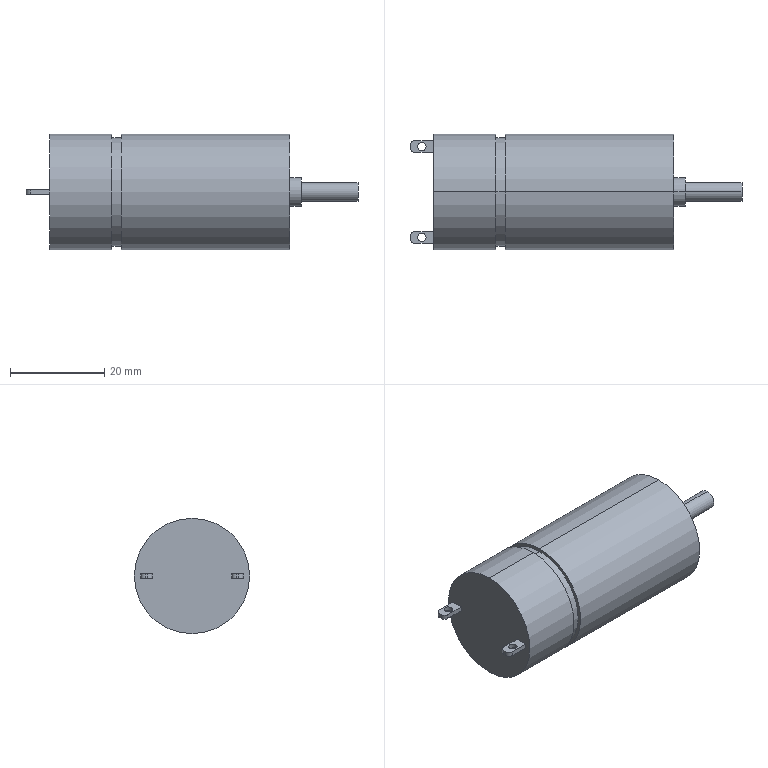Part | SolidWorks | features ICE 4, Extrusion 1, Fillet 1, RevCut 1 | 1 solid | 40 faces | box 70.5 x 24.5 x 24.5 mm | volume 24091 mm3 | cylinder 22 | plane 18 | commonest cylinder face diameters 1.8 x4 2 x4 3.2 x4 24.5 x4 4 x2 6 x2
STEP:
#1=CARTESIAN_POINT('',(46.,0.,-6.9));
#2=VERTEX_POINT('',#1);
#3=CARTESIAN_POINT('',(46.,0.,-10.1));
#4=VERTEX_POINT('',#3);
#5=CARTESIAN_POINT('',(46.,0.,-8.5));
#6=DIRECTION('',(1.,0.,0.));
#7=DIRECTION('',(0.,0.,-1.));
#8=AXIS2_PLACEMENT_3D('',#5,#6,#7);
#9=CIRCLE('',#8,1.6);
#10=EDGE_CURVE('',#2,#4,#9,.T.);
#11=ORIENTED_EDGE('',*,*,#10,.F.);
#12=CARTESIAN_POINT('',(51.,0.,-6.9));
#13=VERTEX_POINT('',#12);
#14=CARTESIAN_POINT('',(46.,0.,-6.9));
#15=DIRECTION('',(1.,0.,0.));
#16=VECTOR('',#15,1000.);
#17=LINE('',#14,#16);
#18=EDGE_CURVE('',#2,#13,#17,.T.);
#19=ORIENTED_EDGE('',*,*,#18,.T.);
#20=CARTESIAN_POINT('',(51.,0.,-10.1));
#21=VERTEX_POINT('',#20);
#22=CARTESIAN_POINT('',(51.,0.,-8.5));
#23=DIRECTION('',(1.,0.,0.));
#24=DIRECTION('',(0.,0.,-1.));
#25=AXIS2_PLACEMENT_3D('',#22,#23,#24);
#26=CIRCLE('',#25,1.6);
#27=EDGE_CURVE('',#13,#21,#26,.T.);
#28=ORIENTED_EDGE('',*,*,#27,.T.);
#29=CARTESIAN_POINT('',(46.,0.,-10.1));
#30=DIRECTION('',(1.,0.,0.));
#31=VECTOR('',#30,1000.);
#32=LINE('',#29,#31);
#33=EDGE_CURVE('',#4,#21,#32,.T.);
#34=ORIENTED_EDGE('',*,*,#33,.F.);
#35=EDGE_LOOP('',(#11,#19,#28,#34));
#36=FACE_OUTER_BOUND('',#35,.T.);
#37=CARTESIAN_POINT('',(46.,0.,-8.5));
#38=DIRECTION('',(1.,0.,0.));
#39=DIRECTION('',(0.,0.,-1.));
#40=AXIS2_PLACEMENT_3D('',#37,#38,#39);
#41=CYLINDRICAL_SURFACE('',#40,1.6);
#42=ADVANCED_FACE('',(#36),#41,.F.);
#43=CARTESIAN_POINT('',(46.,0.,10.1));
#44=VERTEX_POINT('',#43);
#45=CARTESIAN_POINT('',(46.,0.,6.9));
#46=VERTEX_POINT('',#45);
#47=CARTESIAN_POINT('',(46.,0.,8.5));
#48=DIRECTION('',(1.,0.,0.));
#49=DIRECTION('',(0.,0.,-1.));
#50=AXIS2_PLACEMENT_3D('',#47,#48,#49);
#51=CIRCLE('',#50,1.6);
#52=EDGE_CURVE('',#44,#46,#51,.T.);
#53=ORIENTED_EDGE('',*,*,#52,.F.);
#54=CARTESIAN_POINT('',(51.,0.,10.1));
#55=VERTEX_POINT('',#54);
#56=CARTESIAN_POINT('',(46.,0.,10.1));
#57=DIRECTION('',(1.,0.,0.));
#58=VECTOR('',#57,1000.);
#59=LINE('',#56,#58);
#60=EDGE_CURVE('',#44,#55,#59,.T.);
#61=ORIENTED_EDGE('',*,*,#60,.T.);
#62=CARTESIAN_POINT('',(51.,0.,6.9));
#63=VERTEX_POINT('',#62);
#64=CARTESIAN_POINT('',(51.,0.,8.5));
#65=DIRECTION('',(1.,0.,0.));
#66=DIRECTION('',(0.,0.,-1.));
#67=AXIS2_PLACEMENT_3D('',#64,#65,#66);
#68=CIRCLE('',#67,1.6);
#69=EDGE_CURVE('',#55,#63,#68,.T.);
#70=ORIENTED_EDGE('',*,*,#69,.T.);
#71=CARTESIAN_POINT('',(46.,0.,6.9));
#72=DIRECTION('',(1.,0.,0.));
#73=VECTOR('',#72,1000.);
#74=LINE('',#71,#73);
#75=EDGE_CURVE('',#46,#63,#74,.T.);
#76=ORIENTED_EDGE('',*,*,#75,.F.);
#77=EDGE_LOOP('',(#53,#61,#70,#76));
#78=FACE_OUTER_BOUND('',#77,.T.);
#79=CARTESIAN_POINT('',(46.,0.,8.5));
#80=DIRECTION('',(1.,0.,0.));
#81=DIRECTION('',(0.,0.,-1.));
#82=AXIS2_PLACEMENT_3D('',#79,#80,#81);
#83=CYLINDRICAL_SURFACE('',#82,1.6);
#84=ADVANCED_FACE('',(#78),#83,.F.);
#85=CARTESIAN_POINT('',(13.236,0.,-12.25));
#86=VERTEX_POINT('',#85);
#87=CARTESIAN_POINT('',(13.236,0.,12.25));
#88=VERTEX_POINT('',#87);
#89=CARTESIAN_POINT('',(13.236,0.,0.));
#90=DIRECTION('',(1.,0.,0.));
#91=DIRECTION('',(0.,0.,-1.));
#92=AXIS2_PLACEMENT_3D('',#89,#90,#91);
#93=CIRCLE('',#92,12.25);
#94=EDGE_CURVE('',#86,#88,#93,.T.);
#95=ORIENTED_EDGE('',*,*,#94,.F.);
#96=CARTESIAN_POINT('',(0.,0.,-12.25));
#97=VERTEX_POINT('',#96);
#98=CARTESIAN_POINT('',(51.,0.,-12.25));
#99=DIRECTION('',(-1.,0.,0.));
#100=VECTOR('',#99,1000.);
#101=LINE('',#98,#100);
#102=EDGE_CURVE('',#86,#97,#101,.T.);
#103=ORIENTED_EDGE('',*,*,#102,.T.);
#104=CARTESIAN_POINT('',(0.,0.,12.25));
#105=VERTEX_POINT('',#104);
#106=CARTESIAN_POINT('',(0.,0.,0.));
#107=DIRECTION('',(1.,0.,0.));
#108=DIRECTION('',(0.,0.,-1.));
#109=AXIS2_PLACEMENT_3D('',#106,#107,#108);
#110=CIRCLE('',#109,12.25);
#111=EDGE_CURVE('',#97,#105,#110,.T.);
#112=ORIENTED_EDGE('',*,*,#111,.T.);
#113=CARTESIAN_POINT('',(51.,0.,12.25));
#114=DIRECTION('',(-1.,0.,0.));
#115=VECTOR('',#114,1000.);
#116=LINE('',#113,#115);
#117=EDGE_CURVE('',#88,#105,#116,.T.);
#118=ORIENTED_EDGE('',*,*,#117,.F.);
#119=EDGE_LOOP('',(#95,#103,#112,#118));
#120=FACE_OUTER_BOUND('',#119,.T.);
#121=CARTESIAN_POINT('',(51.,0.,0.));
#122=DIRECTION('',(-1.,0.,0.));
#123=DIRECTION('',(0.,0.,1.));
#124=AXIS2_PLACEMENT_3D('',#121,#122,#123);
#125=CYLINDRICAL_SURFACE('',#124,12.25);
#126=ADVANCED_FACE('',(#120),#125,.T.);
#127=CARTESIAN_POINT('',(-3.4,9.654,0.5));
#128=VERTEX_POINT('',#127);
#129=CARTESIAN_POINT('',(-1.6,9.654,0.5));
#130=VERTEX_POINT('',#129);
#131=CARTESIAN_POINT('',(-2.5,9.654,0.5));
#132=DIRECTION('',(0.,0.,1.));
#133=DIRECTION('',(1.,0.,0.));
#134=AXIS2_PLACEMENT_3D('',#131,#132,#133);
#135=CIRCLE('',#134,0.9);
#136=EDGE_CURVE('',#128,#130,#135,.T.);
#137=ORIENTED_EDGE('',*,*,#136,.T.);
#138=CARTESIAN_POINT('',(-1.6,9.654,-0.5));
#139=VERTEX_POINT('',#138);
#140=CARTESIAN_POINT('',(-1.6,9.654,0.5));
#141=DIRECTION('',(0.,0.,-1.));
#142=VECTOR('',#141,1000.);
#143=LINE('',#140,#142);
#144=EDGE_CURVE('',#130,#139,#143,.T.);
#145=ORIENTED_EDGE('',*,*,#144,.T.);
#146=CARTESIAN_POINT('',(-3.4,9.654,-0.5));
#147=VERTEX_POINT('',#146);
#148=CARTESIAN_POINT('',(-2.5,9.654,-0.5));
#149=DIRECTION('',(0.,0.,1.));
#150=DIRECTION('',(1.,0.,0.));
#151=AXIS2_PLACEMENT_3D('',#148,#149,#150);
#152=CIRCLE('',#151,0.9);
#153=EDGE_CURVE('',#147,#139,#152,.T.);
#154=ORIENTED_EDGE('',*,*,#153,.F.);
#155=CARTESIAN_POINT('',(-3.4,9.654,0.5));
#156=DIRECTION('',(0.,0.,-1.));
#157=VECTOR('',#156,1000.);
#158=LINE('',#155,#157);
#159=EDGE_CURVE('',#128,#147,#158,.T.);
#160=ORIENTED_EDGE('',*,*,#159,.F.);
#161=EDGE_LOOP('',(#137,#145,#154,#160));
#162=FACE_OUTER_BOUND('',#161,.T.);
#163=CARTESIAN_POINT('',(-2.5,9.654,0.5));
#164=DIRECTION('',(0.,0.,-1.));
#165=DIRECTION('',(-1.,0.,0.));
#166=AXIS2_PLACEMENT_3D('',#163,#164,#165);
#167=CYLINDRICAL_SURFACE('',#166,0.9);
#168=ADVANCED_FACE('',(#162),#167,.F.);
#169=CARTESIAN_POINT('',(-3.4,-9.654,0.5));
#170=VERTEX_POINT('',#169);
#171=CARTESIAN_POINT('',(-1.6,-9.654,0.5));
#172=VERTEX_POINT('',#171);
#173=CARTESIAN_POINT('',(-2.5,-9.654,0.5));
#174=DIRECTION('',(0.,0.,1.));
#175=DIRECTION('',(-1.,0.,0.));
#176=AXIS2_PLACEMENT_3D('',#173,#174,#175);
#177=CIRCLE('',#176,0.9);
#178=EDGE_CURVE('',#170,#172,#177,.T.);
#179=ORIENTED_EDGE('',*,*,#178,.T.);
#180=CARTESIAN_POINT('',(-1.6,-9.654,-0.5));
#181=VERTEX_POINT('',#180);
#182=CARTESIAN_POINT('',(-1.6,-9.654,0.5));
#183=DIRECTION('',(0.,0.,-1.));
#184=VECTOR('',#183,1000.);
#185=LINE('',#182,#184);
#186=EDGE_CURVE('',#172,#181,#185,.T.);
#187=ORIENTED_EDGE('',*,*,#186,.T.);
#188=CARTESIAN_POINT('',(-3.4,-9.654,-0.5));
#189=VERTEX_POINT('',#188);
#190=CARTESIAN_POINT('',(-2.5,-9.654,-0.5));
#191=DIRECTION('',(0.,0.,1.));
#192=DIRECTION('',(-1.,0.,0.));
#193=AXIS2_PLACEMENT_3D('',#190,#191,#192);
#194=CIRCLE('',#193,0.9);
#195=EDGE_CURVE('',#189,#181,#194,.T.);
#196=ORIENTED_EDGE('',*,*,#195,.F.);
#197=CARTESIAN_POINT('',(-3.4,-9.654,0.5));
#198=DIRECTION('',(0.,0.,-1.));
#199=VECTOR('',#198,1000.);
#200=LINE('',#197,#199);
#201=EDGE_CURVE('',#170,#189,#200,.T.);
#202=ORIENTED_EDGE('',*,*,#201,.F.);
#203=EDGE_LOOP('',(#179,#187,#196,#202));
#204=FACE_OUTER_BOUND('',#203,.T.);
#205=CARTESIAN_POINT('',(-2.5,-9.654,0.5));
#206=DIRECTION('',(0.,0.,-1.));
#207=DIRECTION('',(-1.,0.,0.));
#208=AXIS2_PLACEMENT_3D('',#205,#206,#207);
#209=CYLINDRICAL_SURFACE('',#208,0.9);
#210=ADVANCED_FACE('',(#204),#209,.F.);
#211=CARTESIAN_POINT('',(15.236,0.,11.5));
#212=VERTEX_POINT('',#211);
#213=CARTESIAN_POINT('',(15.236,0.,-11.5));
#214=VERTEX_POINT('',#213);
#215=CARTESIAN_POINT('',(15.236,0.,0.));
#216=DIRECTION('',(-1.,0.,0.));
#217=DIRECTION('',(0.,0.,1.));
#218=AXIS2_PLACEMENT_3D('',#215,#216,#217);
#219=CIRCLE('',#218,11.5);
#220=EDGE_CURVE('',#212,#214,#219,.T.);
#221=ORIENTED_EDGE('',*,*,#220,.T.);
#222=CARTESIAN_POINT('',(13.236,0.,-11.5));
#223=VERTEX_POINT('',#222);
#224=CARTESIAN_POINT('',(-4.366,0.,-11.5));
#225=DIRECTION('',(-1.,0.,0.));
#226=VECTOR('',#225,1000.);
#227=LINE('',#224,#226);
#228=EDGE_CURVE('',#214,#223,#227,.T.);
#229=ORIENTED_EDGE('',*,*,#228,.T.);
#230=CARTESIAN_POINT('',(13.236,0.,11.5));
#231=VERTEX_POINT('',#230);
#232=CARTESIAN_POINT('',(13.236,0.,0.));
#233=DIRECTION('',(-1.,0.,0.));
#234=DIRECTION('',(0.,0.,1.));
#235=AXIS2_PLACEMENT_3D('',#232,#233,#234);
#236=CIRCLE('',#235,11.5);
#237=EDGE_CURVE('',#231,#223,#236,.T.);
#238=ORIENTED_EDGE('',*,*,#237,.F.);
#239=CARTESIAN_POINT('',(-4.366,0.,11.5));
#240=DIRECTION('',(-1.,0.,0.));
#241=VECTOR('',#240,1000.);
#242=LINE('',#239,#241);
#243=EDGE_CURVE('',#212,#231,#242,.T.);
#244=ORIENTED_EDGE('',*,*,#243,.F.);
#245=EDGE_LOOP('',(#221,#229,#238,#244));
#246=FACE_OUTER_BOUND('',#245,.T.);
#247=CARTESIAN_POINT('',(-4.366,0.,0.));
#248=DIRECTION('',(-1.,0.,0.));
#249=DIRECTION('',(0.,0.,1.));
#250=AXIS2_PLACEMENT_3D('',#247,#248,#249);
#251=CYLINDRICAL_SURFACE('',#250,11.5);
#252=ADVANCED_FACE('',(#246),#251,.T.);
#253=CARTESIAN_POINT('',(65.5,0.,-2.));
#254=VERTEX_POINT('',#253);
#255=CARTESIAN_POINT('',(65.5,0.,2.));
#256=VERTEX_POINT('',#255);
#257=CARTESIAN_POINT('',(65.5,0.,0.));
#258=DIRECTION('',(1.,0.,0.));
#259=DIRECTION('',(0.,0.,-1.));
#260=AXIS2_PLACEMENT_3D('',#257,#258,#259);
#261=CIRCLE('',#260,2.);
#262=EDGE_CURVE('',#254,#256,#261,.T.);
#263=ORIENTED_EDGE('',*,*,#262,.F.);
#264=CARTESIAN_POINT('',(53.5,0.,-2.));
#265=VERTEX_POINT('',#264);
#266=CARTESIAN_POINT('',(65.5,0.,-2.));
#267=DIRECTION('',(-1.,0.,0.));
#268=VECTOR('',#267,1000.);
#269=LINE('',#266,#268);
#270=EDGE_CURVE('',#254,#265,#269,.T.);
#271=ORIENTED_EDGE('',*,*,#270,.T.);
#272=CARTESIAN_POINT('',(53.5,0.,2.));
#273=VERTEX_POINT('',#272);
#274=CARTESIAN_POINT('',(53.5,0.,0.));
#275=DIRECTION('',(1.,0.,0.));
#276=DIRECTION('',(0.,0.,-1.));
#277=AXIS2_PLACEMENT_3D('',#274,#275,#276);
#278=CIRCLE('',#277,2.);
#279=EDGE_CURVE('',#265,#273,#278,.T.);
#280=ORIENTED_EDGE('',*,*,#279,.T.);
#281=CARTESIAN_POINT('',(65.5,0.,2.));
#282=DIRECTION('',(-1.,0.,0.));
#283=VECTOR('',#282,1000.);
#284=LINE('',#281,#283);
#285=EDGE_CURVE('',#256,#273,#284,.T.);
#286=ORIENTED_EDGE('',*,*,#285,.F.);
#287=EDGE_LOOP('',(#263,#271,#280,#286));
#288=FACE_OUTER_BOUND('',#287,.T.);
#289=CARTESIAN_POINT('',(65.5,0.,0.));
#290=DIRECTION('',(-1.,0.,0.));
#291=DIRECTION('',(0.,0.,1.));
#292=AXIS2_PLACEMENT_3D('',#289,#290,#291);
#293=CYLINDRICAL_SURFACE('',#292,2.);
#294=ADVANCED_FACE('',(#288),#293,.T.);
#295=CARTESIAN_POINT('',(53.5,0.,-3.));
#296=VERTEX_POINT('',#295);
#297=CARTESIAN_POINT('',(53.5,0.,3.));
#298=VERTEX_POINT('',#297);
#299=CARTESIAN_POINT('',(53.5,0.,0.));
#300=DIRECTION('',(1.,0.,0.));
#301=DIRECTION('',(0.,0.,-1.));
#302=AXIS2_PLACEMENT_3D('',#299,#300,#301);
#303=CIRCLE('',#302,3.);
#304=EDGE_CURVE('',#296,#298,#303,.T.);
#305=ORIENTED_EDGE('',*,*,#304,.F.);
#306=CARTESIAN_POINT('',(51.,0.,-3.));
#307=VERTEX_POINT('',#306);
#308=CARTESIAN_POINT('',(53.5,0.,-3.));
#309=DIRECTION('',(-1.,0.,0.));
#310=VECTOR('',#309,1000.);
#311=LINE('',#308,#310);
#312=EDGE_CURVE('',#296,#307,#311,.T.);
#313=ORIENTED_EDGE('',*,*,#312,.T.);
#314=CARTESIAN_POINT('',(51.,0.,3.));
#315=VERTEX_POINT('',#314);
#316=CARTESIAN_POINT('',(51.,0.,0.));
#317=DIRECTION('',(1.,0.,0.));
#318=DIRECTION('',(0.,0.,-1.));
#319=AXIS2_PLACEMENT_3D('',#316,#317,#318);
#320=CIRCLE('',#319,3.);
#321=EDGE_CURVE('',#307,#315,#320,.T.);
#322=ORIENTED_EDGE('',*,*,#321,.T.);
#323=CARTESIAN_POINT('',(53.5,0.,3.));
#324=DIRECTION('',(-1.,0.,0.));
#325=VECTOR('',#324,1000.);
#326=LINE('',#323,#325);
#327=EDGE_CURVE('',#298,#315,#326,.T.);
#328=ORIENTED_EDGE('',*,*,#327,.F.);
#329=EDGE_LOOP('',(#305,#313,#322,#328));
#330=FACE_OUTER_BOUND('',#329,.T.);
#331=CARTESIAN_POINT('',(53.5,0.,0.));
#332=DIRECTION('',(-1.,0.,0.));
#333=DIRECTION('',(0.,0.,1.));
#334=AXIS2_PLACEMENT_3D('',#331,#332,#333);
#335=CYLINDRICAL_SURFACE('',#334,3.);
#336=ADVANCED_FACE('',(#330),#335,.T.);
#337=CARTESIAN_POINT('',(51.,0.,-12.25));
#338=VERTEX_POINT('',#337);
#339=CARTESIAN_POINT('',(51.,0.,12.25));
#340=VERTEX_POINT('',#339);
#341=CARTESIAN_POINT('',(51.,0.,0.));
#342=DIRECTION('',(1.,0.,0.));
#343=DIRECTION('',(0.,0.,-1.));
#344=AXIS2_PLACEMENT_3D('',#341,#342,#343);
#345=CIRCLE('',#344,12.25);
#346=EDGE_CURVE('',#338,#340,#345,.T.);
#347=ORIENTED_EDGE('',*,*,#346,.F.);
#348=CARTESIAN_POINT('',(15.236,0.,-12.25));
#349=VERTEX_POINT('',#348);
#350=CARTESIAN_POINT('',(51.,0.,-12.25));
#351=DIRECTION('',(-1.,0.,0.));
#352=VECTOR('',#351,1000.);
#353=LINE('',#350,#352);
#354=EDGE_CURVE('',#338,#349,#353,.T.);
#355=ORIENTED_EDGE('',*,*,#354,.T.);
#356=CARTESIAN_POINT('',(15.236,0.,12.25));
#357=VERTEX_POINT('',#356);
#358=CARTESIAN_POINT('',(15.236,0.,0.));
#359=DIRECTION('',(-1.,0.,0.));
#360=DIRECTION('',(0.,0.,1.));
#361=AXIS2_PLACEMENT_3D('',#358,#359,#360);
#362=CIRCLE('',#361,12.25);
#363=EDGE_CURVE('',#357,#349,#362,.T.);
#364=ORIENTED_EDGE('',*,*,#363,.F.);
#365=CARTESIAN_POINT('',(51.,0.,12.25));
#366=DIRECTION('',(-1.,0.,0.));
#367=VECTOR('',#366,1000.);
#368=LINE('',#365,#367);
#369=EDGE_CURVE('',#340,#357,#368,.T.);
#370=ORIENTED_EDGE('',*,*,#369,.F.);
#371=EDGE_LOOP('',(#347,#355,#364,#370));
#372=FACE_OUTER_BOUND('',#371,.T.);
#373=CARTESIAN_POINT('',(51.,0.,0.));
#374=DIRECTION('',(-1.,0.,0.));
#375=DIRECTION('',(0.,0.,1.));
#376=AXIS2_PLACEMENT_3D('',#373,#374,#375);
#377=CYLINDRICAL_SURFACE('',#376,12.25);
#378=ADVANCED_FACE('',(#372),#377,.T.);
#379=ORIENTED_EDGE('',*,*,#354,.F.);
#380=CARTESIAN_POINT('',(51.,0.,0.));
#381=DIRECTION('',(1.,0.,0.));
#382=DIRECTION('',(0.,0.,-1.));
#383=AXIS2_PLACEMENT_3D('',#380,#381,#382);
#384=CIRCLE('',#383,12.25);
#385=EDGE_CURVE('',#340,#338,#384,.T.);
#386=ORIENTED_EDGE('',*,*,#385,.F.);
#387=ORIENTED_EDGE('',*,*,#369,.T.);
#388=CARTESIAN_POINT('',(15.236,0.,0.));
#389=DIRECTION('',(-1.,0.,0.));
#390=DIRECTION('',(0.,0.,1.));
#391=AXIS2_PLACEMENT_3D('',#388,#389,#390);
#392=CIRCLE('',#391,12.25);
#393=EDGE_CURVE('',#349,#357,#392,.T.);
#394=ORIENTED_EDGE('',*,*,#393,.F.);
#395=EDGE_LOOP('',(#379,#386,#387,#394));
#396=FACE_OUTER_BOUND('',#395,.T.);
#397=CARTESIAN_POINT('',(51.,0.,0.));
#398=DIRECTION('',(-1.,0.,0.));
#399=DIRECTION('',(0.,0.,1.));
#400=AXIS2_PLACEMENT_3D('',#397,#398,#399);
#401=CYLINDRICAL_SURFACE('',#400,12.25);
#402=ADVANCED_FACE('',(#396),#401,.T.);
#403=CARTESIAN_POINT('',(53.5,0.,0.));
#404=DIRECTION('',(1.,0.,0.));
#405=DIRECTION('',(0.,0.,-1.));
#406=AXIS2_PLACEMENT_3D('',#403,#404,#405);
#407=CIRCLE('',#406,3.);
#408=EDGE_CURVE('',#298,#296,#407,.T.);
#409=ORIENTED_EDGE('',*,*,#408,.T.);
#410=ORIENTED_EDGE('',*,*,#304,.T.);
#411=EDGE_LOOP('',(#409,#410));
#412=FACE_OUTER_BOUND('',#411,.T.);
#413=CARTESIAN_POINT('',(53.5,0.,0.));
#414=DIRECTION('',(1.,0.,0.));
#415=DIRECTION('',(0.,0.,-1.));
#416=AXIS2_PLACEMENT_3D('',#413,#414,#415);
#417=CIRCLE('',#416,2.);
#418=EDGE_CURVE('',#273,#265,#417,.T.);
#419=ORIENTED_EDGE('',*,*,#418,.F.);
#420=ORIENTED_EDGE('',*,*,#279,.F.);
#421=EDGE_LOOP('',(#419,#420));
#422=FACE_BOUND('',#421,.T.);
#423=CARTESIAN_POINT('',(53.5,0.,0.));
#424=DIRECTION('',(1.,0.,0.));
#425=DIRECTION('',(0.,0.,-1.));
#426=AXIS2_PLACEMENT_3D('',#423,#424,#425);
#427=PLANE('',#426);
#428=ADVANCED_FACE('',(#412,#422),#427,.T.);
#429=CARTESIAN_POINT('',(51.,0.,-8.5));
#430=DIRECTION('',(1.,0.,0.));
#431=DIRECTION('',(0.,0.,-1.));
#432=AXIS2_PLACEMENT_3D('',#429,#430,#431);
#433=CIRCLE('',#432,1.6);
#434=EDGE_CURVE('',#21,#13,#433,.T.);
#435=ORIENTED_EDGE('',*,*,#434,.F.);
#436=ORIENTED_EDGE('',*,*,#27,.F.);
#437=EDGE_LOOP('',(#435,#436));
#438=FACE_BOUND('',#437,.T.);
#439=CARTESIAN_POINT('',(51.,0.,8.5));
#440=DIRECTION('',(1.,0.,0.));
#441=DIRECTION('',(0.,0.,-1.));
#442=AXIS2_PLACEMENT_3D('',#439,#440,#441);
#443=CIRCLE('',#442,1.6);
#444=EDGE_CURVE('',#63,#55,#443,.T.);
#445=ORIENTED_EDGE('',*,*,#444,.F.);
#446=ORIENTED_EDGE('',*,*,#69,.F.);
#447=EDGE_LOOP('',(#445,#446));
#448=FACE_BOUND('',#447,.T.);
#449=ORIENTED_EDGE('',*,*,#385,.T.);
#450=ORIENTED_EDGE('',*,*,#346,.T.);
#451=EDGE_LOOP('',(#449,#450));
#452=FACE_OUTER_BOUND('',#451,.T.);
#453=CARTESIAN_POINT('',(51.,0.,0.));
#454=DIRECTION('',(1.,0.,0.));
#455=DIRECTION('',(0.,0.,-1.));
#456=AXIS2_PLACEMENT_3D('',#453,#454,#455);
#457=CIRCLE('',#456,3.);
#458=EDGE_CURVE('',#315,#307,#457,.T.);
#459=ORIENTED_EDGE('',*,*,#458,.F.);
#460=ORIENTED_EDGE('',*,*,#321,.F.);
#461=EDGE_LOOP('',(#459,#460));
#462=FACE_BOUND('',#461,.T.);
#463=CARTESIAN_POINT('',(51.,0.,0.));
#464=DIRECTION('',(1.,0.,0.));
#465=DIRECTION('',(0.,0.,-1.));
#466=AXIS2_PLACEMENT_3D('',#463,#464,#465);
#467=PLANE('',#466);
#468=ADVANCED_FACE('',(#438,#448,#452,#462),#467,.T.);
#469=ORIENTED_EDGE('',*,*,#312,.F.);
#470=ORIENTED_EDGE('',*,*,#408,.F.);
#471=ORIENTED_EDGE('',*,*,#327,.T.);
#472=ORIENTED_EDGE('',*,*,#458,.T.);
#473=EDGE_LOOP('',(#469,#470,#471,#472));
#474=FACE_OUTER_BOUND('',#473,.T.);
#475=CARTESIAN_POINT('',(53.5,0.,0.));
#476=DIRECTION('',(-1.,0.,0.));
#477=DIRECTION('',(0.,0.,1.));
#478=AXIS2_PLACEMENT_3D('',#475,#476,#477);
#479=CYLINDRICAL_SURFACE('',#478,3.);
#480=ADVANCED_FACE('',(#474),#479,.T.);
#481=ORIENTED_EDGE('',*,*,#270,.F.);
#482=CARTESIAN_POINT('',(65.5,0.,0.));
#483=DIRECTION('',(1.,0.,0.));
#484=DIRECTION('',(0.,0.,-1.));
#485=AXIS2_PLACEMENT_3D('',#482,#483,#484);
#486=CIRCLE('',#485,2.);
#487=EDGE_CURVE('',#256,#254,#486,.T.);
#488=ORIENTED_EDGE('',*,*,#487,.F.);
#489=ORIENTED_EDGE('',*,*,#285,.T.);
#490=ORIENTED_EDGE('',*,*,#418,.T.);
#491=EDGE_LOOP('',(#481,#488,#489,#490));
#492=FACE_OUTER_BOUND('',#491,.T.);
#493=CARTESIAN_POINT('',(65.5,0.,0.));
#494=DIRECTION('',(-1.,0.,0.));
#495=DIRECTION('',(0.,0.,1.));
#496=AXIS2_PLACEMENT_3D('',#493,#494,#495);
#497=CYLINDRICAL_SURFACE('',#496,2.);
#498=ADVANCED_FACE('',(#492),#497,.T.);
#499=ORIENTED_EDGE('',*,*,#487,.T.);
#500=ORIENTED_EDGE('',*,*,#262,.T.);
#501=EDGE_LOOP('',(#499,#500));
#502=FACE_OUTER_BOUND('',#501,.T.);
#503=CARTESIAN_POINT('',(65.5,0.,0.));
#504=DIRECTION('',(1.,0.,0.));
#505=DIRECTION('',(0.,0.,-1.));
#506=AXIS2_PLACEMENT_3D('',#503,#504,#505);
#507=PLANE('',#506);
#508=ADVANCED_FACE('',(#502),#507,.T.);
#509=ORIENTED_EDGE('',*,*,#220,.F.);
#510=CARTESIAN_POINT('',(15.236,0.,0.));
#511=DIRECTION('',(-1.,0.,0.));
#512=DIRECTION('',(0.,0.,1.));
#513=AXIS2_PLACEMENT_3D('',#510,#511,#512);
#514=CIRCLE('',#513,11.5);
#515=EDGE_CURVE('',#214,#212,#514,.T.);
#516=ORIENTED_EDGE('',*,*,#515,.F.);
#517=EDGE_LOOP('',(#509,#516));
#518=FACE_BOUND('',#517,.T.);
#519=ORIENTED_EDGE('',*,*,#363,.T.);
#520=ORIENTED_EDGE('',*,*,#393,.T.);
#521=EDGE_LOOP('',(#519,#520));
#522=FACE_OUTER_BOUND('',#521,.T.);
#523=CARTESIAN_POINT('',(15.236,15.,0.));
#524=DIRECTION('',(-1.,0.,0.));
#525=DIRECTION('',(0.,0.,1.));
#526=AXIS2_PLACEMENT_3D('',#523,#524,#525);
#527=PLANE('',#526);
#528=ADVANCED_FACE('',(#518,#522),#527,.T.);
#529=ORIENTED_EDGE('',*,*,#237,.T.);
#530=CARTESIAN_POINT('',(13.236,0.,0.));
#531=DIRECTION('',(-1.,0.,0.));
#532=DIRECTION('',(0.,0.,1.));
#533=AXIS2_PLACEMENT_3D('',#530,#531,#532);
#534=CIRCLE('',#533,11.5);
#535=EDGE_CURVE('',#223,#231,#534,.T.);
#536=ORIENTED_EDGE('',*,*,#535,.T.);
#537=EDGE_LOOP('',(#529,#536));
#538=FACE_BOUND('',#537,.T.);
#539=CARTESIAN_POINT('',(13.236,0.,0.));
#540=DIRECTION('',(1.,0.,0.));
#541=DIRECTION('',(0.,0.,-1.));
#542=AXIS2_PLACEMENT_3D('',#539,#540,#541);
#543=CIRCLE('',#542,12.25);
#544=EDGE_CURVE('',#88,#86,#543,.T.);
#545=ORIENTED_EDGE('',*,*,#544,.T.);
#546=ORIENTED_EDGE('',*,*,#94,.T.);
#547=EDGE_LOOP('',(#545,#546));
#548=FACE_OUTER_BOUND('',#547,.T.);
#549=CARTESIAN_POINT('',(13.236,15.,0.));
#550=DIRECTION('',(1.,0.,0.));
#551=DIRECTION('',(0.,0.,-1.));
#552=AXIS2_PLACEMENT_3D('',#549,#550,#551);
#553=PLANE('',#552);
#554=ADVANCED_FACE('',(#538,#548),#553,.T.);
#555=ORIENTED_EDGE('',*,*,#228,.F.);
#556=ORIENTED_EDGE('',*,*,#515,.T.);
#557=ORIENTED_EDGE('',*,*,#243,.T.);
#558=ORIENTED_EDGE('',*,*,#535,.F.);
#559=EDGE_LOOP('',(#555,#556,#557,#558));
#560=FACE_OUTER_BOUND('',#559,.T.);
#561=CARTESIAN_POINT('',(-4.366,0.,0.));
#562=DIRECTION('',(-1.,0.,0.));
#563=DIRECTION('',(0.,0.,1.));
#564=AXIS2_PLACEMENT_3D('',#561,#562,#563);
#565=CYLINDRICAL_SURFACE('',#564,11.5);
#566=ADVANCED_FACE('',(#560),#565,.T.);
#567=ORIENTED_EDGE('',*,*,#186,.F.);
#568=CARTESIAN_POINT('',(-2.5,-9.654,0.5));
#569=DIRECTION('',(0.,0.,1.));
#570=DIRECTION('',(-1.,0.,0.));
#571=AXIS2_PLACEMENT_3D('',#568,#569,#570);
#572=CIRCLE('',#571,0.9);
#573=EDGE_CURVE('',#172,#170,#572,.T.);
#574=ORIENTED_EDGE('',*,*,#573,.T.);
#575=ORIENTED_EDGE('',*,*,#201,.T.);
#576=CARTESIAN_POINT('',(-2.5,-9.654,-0.5));
#577=DIRECTION('',(0.,0.,1.));
#578=DIRECTION('',(-1.,0.,0.));
#579=AXIS2_PLACEMENT_3D('',#576,#577,#578);
#580=CIRCLE('',#579,0.9);
#581=EDGE_CURVE('',#181,#189,#580,.T.);
#582=ORIENTED_EDGE('',*,*,#581,.F.);
#583=EDGE_LOOP('',(#567,#574,#575,#582));
#584=FACE_OUTER_BOUND('',#583,.T.);
#585=CARTESIAN_POINT('',(-2.5,-9.654,0.5));
#586=DIRECTION('',(0.,0.,-1.));
#587=DIRECTION('',(-1.,0.,0.));
#588=AXIS2_PLACEMENT_3D('',#585,#586,#587);
#589=CYLINDRICAL_SURFACE('',#588,0.9);
#590=ADVANCED_FACE('',(#584),#589,.F.);
#591=CARTESIAN_POINT('',(-4.,-8.404,0.5));
#592=VERTEX_POINT('',#591);
#593=CARTESIAN_POINT('',(-5.,-9.404,0.5));
#594=VERTEX_POINT('',#593);
#595=CARTESIAN_POINT('',(-4.,-9.404,0.5));
#596=DIRECTION('',(0.,0.,1.));
#597=DIRECTION('',(-1.,0.,0.));
#598=AXIS2_PLACEMENT_3D('',#595,#596,#597);
#599=CIRCLE('',#598,1.);
#600=EDGE_CURVE('',#592,#594,#599,.T.);
#601=ORIENTED_EDGE('',*,*,#600,.F.);
#602=CARTESIAN_POINT('',(-4.,-8.404,-0.5));
#603=VERTEX_POINT('',#602);
#604=CARTESIAN_POINT('',(-4.,-8.404,0.5));
#605=DIRECTION('',(0.,0.,1.));
#606=VECTOR('',#605,1000.);
#607=LINE('',#604,#606);
#608=EDGE_CURVE('',#603,#592,#607,.T.);
#609=ORIENTED_EDGE('',*,*,#608,.F.);
#610=CARTESIAN_POINT('',(-5.,-9.404,-0.5));
#611=VERTEX_POINT('',#610);
#612=CARTESIAN_POINT('',(-4.,-9.404,-0.5));
#613=DIRECTION('',(0.,0.,-1.));
#614=DIRECTION('',(-1.,0.,0.));
#615=AXIS2_PLACEMENT_3D('',#612,#613,#614);
#616=CIRCLE('',#615,1.);
#617=EDGE_CURVE('',#611,#603,#616,.T.);
#618=ORIENTED_EDGE('',*,*,#617,.F.);
#619=CARTESIAN_POINT('',(-5.,-9.404,0.5));
#620=DIRECTION('',(0.,0.,-1.));
#621=VECTOR('',#620,1000.);
#622=LINE('',#619,#621);
#623=EDGE_CURVE('',#594,#611,#622,.T.);
#624=ORIENTED_EDGE('',*,*,#623,.F.);
#625=EDGE_LOOP('',(#601,#609,#618,#624));
#626=FACE_OUTER_BOUND('',#625,.T.);
#627=CARTESIAN_POINT('',(-4.,-9.404,0.5));
#628=DIRECTION('',(0.,0.,-1.));
#629=DIRECTION('',(-1.,0.,0.));
#630=AXIS2_PLACEMENT_3D('',#627,#628,#629);
#631=CYLINDRICAL_SURFACE('',#630,1.);
#632=ADVANCED_FACE('',(#626),#631,.T.);
#633=CARTESIAN_POINT('',(-5.,-9.904,0.5));
#634=VERTEX_POINT('',#633);
#635=CARTESIAN_POINT('',(-5.,-10.904,0.5));
#636=DIRECTION('',(0.,-1.,0.));
#637=VECTOR('',#636,1000.);
#638=LINE('',#635,#637);
#639=EDGE_CURVE('',#594,#634,#638,.T.);
#640=ORIENTED_EDGE('',*,*,#639,.F.);
#641=ORIENTED_EDGE('',*,*,#623,.T.);
#642=CARTESIAN_POINT('',(-5.,-9.904,-0.5));
#643=VERTEX_POINT('',#642);
#644=CARTESIAN_POINT('',(-5.,-10.904,-0.5));
#645=DIRECTION('',(0.,-1.,0.));
#646=VECTOR('',#645,1000.);
#647=LINE('',#644,#646);
#648=EDGE_CURVE('',#611,#643,#647,.T.);
#649=ORIENTED_EDGE('',*,*,#648,.T.);
#650=CARTESIAN_POINT('',(-5.,-9.904,0.5));
#651=DIRECTION('',(0.,0.,1.));
#652=VECTOR('',#651,1000.);
#653=LINE('',#650,#652);
#654=EDGE_CURVE('',#643,#634,#653,.T.);
#655=ORIENTED_EDGE('',*,*,#654,.T.);
#656=EDGE_LOOP('',(#640,#641,#649,#655));
#657=FACE_OUTER_BOUND('',#656,.T.);
#658=CARTESIAN_POINT('',(-5.,-10.904,0.5));
#659=DIRECTION('',(1.,0.,0.));
#660=DIRECTION('',(0.,1.,0.));
#661=AXIS2_PLACEMENT_3D('',#658,#659,#660);
#662=PLANE('',#661);
#663=ADVANCED_FACE('',(#657),#662,.F.);
#664=CARTESIAN_POINT('',(-4.,-10.904,0.5));
#665=VERTEX_POINT('',#664);
#666=CARTESIAN_POINT('',(-4.,-9.904,0.5));
#667=DIRECTION('',(0.,0.,1.));
#668=DIRECTION('',(-1.,0.,0.));
#669=AXIS2_PLACEMENT_3D('',#666,#667,#668);
#670=CIRCLE('',#669,1.);
#671=EDGE_CURVE('',#634,#665,#670,.T.);
#672=ORIENTED_EDGE('',*,*,#671,.F.);
#673=ORIENTED_EDGE('',*,*,#654,.F.);
#674=CARTESIAN_POINT('',(-4.,-10.904,-0.5));
#675=VERTEX_POINT('',#674);
#676=CARTESIAN_POINT('',(-4.,-9.904,-0.5));
#677=DIRECTION('',(0.,0.,-1.));
#678=DIRECTION('',(-1.,0.,0.));
#679=AXIS2_PLACEMENT_3D('',#676,#677,#678);
#680=CIRCLE('',#679,1.);
#681=EDGE_CURVE('',#675,#643,#680,.T.);
#682=ORIENTED_EDGE('',*,*,#681,.F.);
#683=CARTESIAN_POINT('',(-4.,-10.904,0.5));
#684=DIRECTION('',(0.,0.,-1.));
#685=VECTOR('',#684,1000.);
#686=LINE('',#683,#685);
#687=EDGE_CURVE('',#665,#675,#686,.T.);
#688=ORIENTED_EDGE('',*,*,#687,.F.);
#689=EDGE_LOOP('',(#672,#673,#682,#688));
#690=FACE_OUTER_BOUND('',#689,.T.);
#691=CARTESIAN_POINT('',(-4.,-9.904,0.5));
#692=DIRECTION('',(0.,0.,-1.));
#693=DIRECTION('',(-1.,0.,0.));
#694=AXIS2_PLACEMENT_3D('',#691,#692,#693);
#695=CYLINDRICAL_SURFACE('',#694,1.);
#696=ADVANCED_FACE('',(#690),#695,.T.);
#697=ORIENTED_EDGE('',*,*,#144,.F.);
#698=CARTESIAN_POINT('',(-2.5,9.654,0.5));
#699=DIRECTION('',(0.,0.,1.));
#700=DIRECTION('',(1.,0.,0.));
#701=AXIS2_PLACEMENT_3D('',#698,#699,#700);
#702=CIRCLE('',#701,0.9);
#703=EDGE_CURVE('',#130,#128,#702,.T.);
#704=ORIENTED_EDGE('',*,*,#703,.T.);
#705=ORIENTED_EDGE('',*,*,#159,.T.);
#706=CARTESIAN_POINT('',(-2.5,9.654,-0.5));
#707=DIRECTION('',(0.,0.,1.));
#708=DIRECTION('',(1.,0.,0.));
#709=AXIS2_PLACEMENT_3D('',#706,#707,#708);
#710=CIRCLE('',#709,0.9);
#711=EDGE_CURVE('',#139,#147,#710,.T.);
#712=ORIENTED_EDGE('',*,*,#711,.F.);
#713=EDGE_LOOP('',(#697,#704,#705,#712));
#714=FACE_OUTER_BOUND('',#713,.T.);
#715=CARTESIAN_POINT('',(-2.5,9.654,0.5));
#716=DIRECTION('',(0.,0.,-1.));
#717=DIRECTION('',(-1.,0.,0.));
#718=AXIS2_PLACEMENT_3D('',#715,#716,#717);
#719=CYLINDRICAL_SURFACE('',#718,0.9);
#720=ADVANCED_FACE('',(#714),#719,.F.);
#721=CARTESIAN_POINT('',(-5.,9.404,0.5));
#722=VERTEX_POINT('',#721);
#723=CARTESIAN_POINT('',(-4.,8.404,0.5));
#724=VERTEX_POINT('',#723);
#725=CARTESIAN_POINT('',(-4.,9.404,0.5));
#726=DIRECTION('',(0.,0.,1.));
#727=DIRECTION('',(1.,0.,0.));
#728=AXIS2_PLACEMENT_3D('',#725,#726,#727);
#729=CIRCLE('',#728,1.);
#730=EDGE_CURVE('',#722,#724,#729,.T.);
#731=ORIENTED_EDGE('',*,*,#730,.F.);
#732=CARTESIAN_POINT('',(-5.,9.404,-0.5));
#733=VERTEX_POINT('',#732);
#734=CARTESIAN_POINT('',(-5.,9.404,0.5));
#735=DIRECTION('',(0.,0.,1.));
#736=VECTOR('',#735,1000.);
#737=LINE('',#734,#736);
#738=EDGE_CURVE('',#733,#722,#737,.T.);
#739=ORIENTED_EDGE('',*,*,#738,.F.);
#740=CARTESIAN_POINT('',(-4.,8.404,-0.5));
#741=VERTEX_POINT('',#740);
#742=CARTESIAN_POINT('',(-4.,9.404,-0.5));
#743=DIRECTION('',(0.,0.,-1.));
#744=DIRECTION('',(1.,0.,0.));
#745=AXIS2_PLACEMENT_3D('',#742,#743,#744);
#746=CIRCLE('',#745,1.);
#747=EDGE_CURVE('',#741,#733,#746,.T.);
#748=ORIENTED_EDGE('',*,*,#747,.F.);
#749=CARTESIAN_POINT('',(-4.,8.404,0.5));
#750=DIRECTION('',(0.,0.,-1.));
#751=VECTOR('',#750,1000.);
#752=LINE('',#749,#751);
#753=EDGE_CURVE('',#724,#741,#752,.T.);
#754=ORIENTED_EDGE('',*,*,#753,.F.);
#755=EDGE_LOOP('',(#731,#739,#748,#754));
#756=FACE_OUTER_BOUND('',#755,.T.);
#757=CARTESIAN_POINT('',(-4.,9.404,0.5));
#758=DIRECTION('',(0.,0.,-1.));
#759=DIRECTION('',(-1.,0.,0.));
#760=AXIS2_PLACEMENT_3D('',#757,#758,#759);
#761=CYLINDRICAL_SURFACE('',#760,1.);
#762=ADVANCED_FACE('',(#756),#761,.T.);
#763=CARTESIAN_POINT('',(-5.,9.904,-0.5));
#764=VERTEX_POINT('',#763);
#765=CARTESIAN_POINT('',(-5.,10.904,-0.5));
#766=DIRECTION('',(0.,-1.,0.));
#767=VECTOR('',#766,1000.);
#768=LINE('',#765,#767);
#769=EDGE_CURVE('',#764,#733,#768,.T.);
#770=ORIENTED_EDGE('',*,*,#769,.T.);
#771=ORIENTED_EDGE('',*,*,#738,.T.);
#772=CARTESIAN_POINT('',(-5.,9.904,0.5));
#773=VERTEX_POINT('',#772);
#774=CARTESIAN_POINT('',(-5.,10.904,0.5));
#775=DIRECTION('',(0.,-1.,0.));
#776=VECTOR('',#775,1000.);
#777=LINE('',#774,#776);
#778=EDGE_CURVE('',#773,#722,#777,.T.);
#779=ORIENTED_EDGE('',*,*,#778,.F.);
#780=CARTESIAN_POINT('',(-5.,9.904,0.5));
#781=DIRECTION('',(0.,0.,-1.));
#782=VECTOR('',#781,1000.);
#783=LINE('',#780,#782);
#784=EDGE_CURVE('',#773,#764,#783,.T.);
#785=ORIENTED_EDGE('',*,*,#784,.T.);
#786=EDGE_LOOP('',(#770,#771,#779,#785));
#787=FACE_OUTER_BOUND('',#786,.T.);
#788=CARTESIAN_POINT('',(-5.,10.904,0.5));
#789=DIRECTION('',(1.,0.,0.));
#790=DIRECTION('',(0.,1.,0.));
#791=AXIS2_PLACEMENT_3D('',#788,#789,#790);
#792=PLANE('',#791);
#793=ADVANCED_FACE('',(#787),#792,.F.);
#794=CARTESIAN_POINT('',(-4.,10.904,0.5));
#795=VERTEX_POINT('',#794);
#796=CARTESIAN_POINT('',(-4.,9.904,0.5));
#797=DIRECTION('',(0.,0.,1.));
#798=DIRECTION('',(1.,0.,0.));
#799=AXIS2_PLACEMENT_3D('',#796,#797,#798);
#800=CIRCLE('',#799,1.);
#801=EDGE_CURVE('',#795,#773,#800,.T.);
#802=ORIENTED_EDGE('',*,*,#801,.F.);
#803=CARTESIAN_POINT('',(-4.,10.904,-0.5));
#804=VERTEX_POINT('',#803);
#805=CARTESIAN_POINT('',(-4.,10.904,0.5));
#806=DIRECTION('',(0.,0.,1.));
#807=VECTOR('',#806,1000.);
#808=LINE('',#805,#807);
#809=EDGE_CURVE('',#804,#795,#808,.T.);
#810=ORIENTED_EDGE('',*,*,#809,.F.);
#811=CARTESIAN_POINT('',(-4.,9.904,-0.5));
#812=DIRECTION('',(0.,0.,-1.));
#813=DIRECTION('',(1.,0.,0.));
#814=AXIS2_PLACEMENT_3D('',#811,#812,#813);
#815=CIRCLE('',#814,1.);
#816=EDGE_CURVE('',#764,#804,#815,.T.);
#817=ORIENTED_EDGE('',*,*,#816,.F.);
#818=ORIENTED_EDGE('',*,*,#784,.F.);
#819=EDGE_LOOP('',(#802,#810,#817,#818));
#820=FACE_OUTER_BOUND('',#819,.T.);
#821=CARTESIAN_POINT('',(-4.,9.904,0.5));
#822=DIRECTION('',(0.,0.,-1.));
#823=DIRECTION('',(-1.,0.,0.));
#824=AXIS2_PLACEMENT_3D('',#821,#822,#823);
#825=CYLINDRICAL_SURFACE('',#824,1.);
#826=ADVANCED_FACE('',(#820),#825,.T.);
#827=CARTESIAN_POINT('',(0.,-8.404,0.5));
#828=VERTEX_POINT('',#827);
#829=CARTESIAN_POINT('',(-5.,-8.404,0.5));
#830=DIRECTION('',(-1.,0.,0.));
#831=VECTOR('',#830,1000.);
#832=LINE('',#829,#831);
#833=EDGE_CURVE('',#828,#592,#832,.T.);
#834=ORIENTED_EDGE('',*,*,#833,.T.);
#835=ORIENTED_EDGE('',*,*,#600,.T.);
#836=ORIENTED_EDGE('',*,*,#639,.T.);
#837=ORIENTED_EDGE('',*,*,#671,.T.);
#838=CARTESIAN_POINT('',(0.,-10.904,0.5));
#839=VERTEX_POINT('',#838);
#840=CARTESIAN_POINT('',(-5.,-10.904,0.5));
#841=DIRECTION('',(1.,0.,0.));
#842=VECTOR('',#841,1000.);
#843=LINE('',#840,#842);
#844=EDGE_CURVE('',#665,#839,#843,.T.);
#845=ORIENTED_EDGE('',*,*,#844,.T.);
#846=CARTESIAN_POINT('',(0.,-10.904,0.5));
#847=DIRECTION('',(0.,1.,0.));
#848=VECTOR('',#847,1000.);
#849=LINE('',#846,#848);
#850=EDGE_CURVE('',#839,#828,#849,.T.);
#851=ORIENTED_EDGE('',*,*,#850,.T.);
#852=EDGE_LOOP('',(#834,#835,#836,#837,#845,#851));
#853=FACE_OUTER_BOUND('',#852,.T.);
#854=ORIENTED_EDGE('',*,*,#178,.F.);
#855=ORIENTED_EDGE('',*,*,#573,.F.);
#856=EDGE_LOOP('',(#854,#855));
#857=FACE_BOUND('',#856,.T.);
#858=CARTESIAN_POINT('',(0.,0.,0.5));
#859=DIRECTION('',(0.,0.,-1.));
#860=DIRECTION('',(-1.,0.,0.));
#861=AXIS2_PLACEMENT_3D('',#858,#859,#860);
#862=PLANE('',#861);
#863=ADVANCED_FACE('',(#853,#857),#862,.F.);
#864=CARTESIAN_POINT('',(0.,-8.404,-0.5));
#865=VERTEX_POINT('',#864);
#866=CARTESIAN_POINT('',(-5.,-8.404,-0.5));
#867=DIRECTION('',(-1.,0.,0.));
#868=VECTOR('',#867,1000.);
#869=LINE('',#866,#868);
#870=EDGE_CURVE('',#865,#603,#869,.T.);
#871=ORIENTED_EDGE('',*,*,#870,.T.);
#872=ORIENTED_EDGE('',*,*,#608,.T.);
#873=ORIENTED_EDGE('',*,*,#833,.F.);
#874=CARTESIAN_POINT('',(0.,-8.404,0.5));
#875=DIRECTION('',(0.,0.,-1.));
#876=VECTOR('',#875,1000.);
#877=LINE('',#874,#876);
#878=EDGE_CURVE('',#828,#865,#877,.T.);
#879=ORIENTED_EDGE('',*,*,#878,.T.);
#880=EDGE_LOOP('',(#871,#872,#873,#879));
#881=FACE_OUTER_BOUND('',#880,.T.);
#882=CARTESIAN_POINT('',(-5.,-8.404,0.5));
#883=DIRECTION('',(0.,-1.,0.));
#884=DIRECTION('',(0.,0.,-1.));
#885=AXIS2_PLACEMENT_3D('',#882,#883,#884);
#886=PLANE('',#885);
#887=ADVANCED_FACE('',(#881),#886,.F.);
#888=ORIENTED_EDGE('',*,*,#648,.F.);
#889=ORIENTED_EDGE('',*,*,#617,.T.);
#890=ORIENTED_EDGE('',*,*,#870,.F.);
#891=CARTESIAN_POINT('',(0.,-10.904,-0.5));
#892=VERTEX_POINT('',#891);
#893=CARTESIAN_POINT('',(0.,-10.904,-0.5));
#894=DIRECTION('',(0.,1.,0.));
#895=VECTOR('',#894,1000.);
#896=LINE('',#893,#895);
#897=EDGE_CURVE('',#892,#865,#896,.T.);
#898=ORIENTED_EDGE('',*,*,#897,.F.);
#899=CARTESIAN_POINT('',(-5.,-10.904,-0.5));
#900=DIRECTION('',(1.,0.,0.));
#901=VECTOR('',#900,1000.);
#902=LINE('',#899,#901);
#903=EDGE_CURVE('',#675,#892,#902,.T.);
#904=ORIENTED_EDGE('',*,*,#903,.F.);
#905=ORIENTED_EDGE('',*,*,#681,.T.);
#906=EDGE_LOOP('',(#888,#889,#890,#898,#904,#905));
#907=FACE_OUTER_BOUND('',#906,.T.);
#908=ORIENTED_EDGE('',*,*,#195,.T.);
#909=ORIENTED_EDGE('',*,*,#581,.T.);
#910=EDGE_LOOP('',(#908,#909));
#911=FACE_BOUND('',#910,.T.);
#912=CARTESIAN_POINT('',(0.,0.,-0.5));
#913=DIRECTION('',(0.,0.,-1.));
#914=DIRECTION('',(-1.,0.,0.));
#915=AXIS2_PLACEMENT_3D('',#912,#913,#914);
#916=PLANE('',#915);
#917=ADVANCED_FACE('',(#907,#911),#916,.T.);
#918=ORIENTED_EDGE('',*,*,#844,.F.);
#919=ORIENTED_EDGE('',*,*,#687,.T.);
#920=ORIENTED_EDGE('',*,*,#903,.T.);
#921=CARTESIAN_POINT('',(0.,-10.904,0.5));
#922=DIRECTION('',(0.,0.,-1.));
#923=VECTOR('',#922,1000.);
#924=LINE('',#921,#923);
#925=EDGE_CURVE('',#839,#892,#924,.T.);
#926=ORIENTED_EDGE('',*,*,#925,.F.);
#927=EDGE_LOOP('',(#918,#919,#920,#926));
#928=FACE_OUTER_BOUND('',#927,.T.);
#929=CARTESIAN_POINT('',(-5.,-10.904,0.5));
#930=DIRECTION('',(0.,1.,0.));
#931=DIRECTION('',(0.,0.,1.));
#932=AXIS2_PLACEMENT_3D('',#929,#930,#931);
#933=PLANE('',#932);
#934=ADVANCED_FACE('',(#928),#933,.F.);
#935=CARTESIAN_POINT('',(0.,8.404,-0.5));
#936=VERTEX_POINT('',#935);
#937=CARTESIAN_POINT('',(-5.,8.404,-0.5));
#938=DIRECTION('',(1.,0.,0.));
#939=VECTOR('',#938,1000.);
#940=LINE('',#937,#939);
#941=EDGE_CURVE('',#741,#936,#940,.T.);
#942=ORIENTED_EDGE('',*,*,#941,.F.);
#943=ORIENTED_EDGE('',*,*,#747,.T.);
#944=ORIENTED_EDGE('',*,*,#769,.F.);
#945=ORIENTED_EDGE('',*,*,#816,.T.);
#946=CARTESIAN_POINT('',(0.,10.904,-0.5));
#947=VERTEX_POINT('',#946);
#948=CARTESIAN_POINT('',(-5.,10.904,-0.5));
#949=DIRECTION('',(-1.,0.,0.));
#950=VECTOR('',#949,1000.);
#951=LINE('',#948,#950);
#952=EDGE_CURVE('',#947,#804,#951,.T.);
#953=ORIENTED_EDGE('',*,*,#952,.F.);
#954=CARTESIAN_POINT('',(0.,10.904,-0.5));
#955=DIRECTION('',(0.,1.,0.));
#956=VECTOR('',#955,1000.);
#957=LINE('',#954,#956);
#958=EDGE_CURVE('',#936,#947,#957,.T.);
#959=ORIENTED_EDGE('',*,*,#958,.F.);
#960=EDGE_LOOP('',(#942,#943,#944,#945,#953,#959));
#961=FACE_OUTER_BOUND('',#960,.T.);
#962=ORIENTED_EDGE('',*,*,#153,.T.);
#963=ORIENTED_EDGE('',*,*,#711,.T.);
#964=EDGE_LOOP('',(#962,#963));
#965=FACE_BOUND('',#964,.T.);
#966=CARTESIAN_POINT('',(0.,0.,-0.5));
#967=DIRECTION('',(0.,0.,1.));
#968=DIRECTION('',(1.,0.,0.));
#969=AXIS2_PLACEMENT_3D('',#966,#967,#968);
#970=PLANE('',#969);
#971=ADVANCED_FACE('',(#961,#965),#970,.F.);
#972=CARTESIAN_POINT('',(0.,8.404,0.5));
#973=VERTEX_POINT('',#972);
#974=CARTESIAN_POINT('',(-5.,8.404,0.5));
#975=DIRECTION('',(1.,0.,0.));
#976=VECTOR('',#975,1000.);
#977=LINE('',#974,#976);
#978=EDGE_CURVE('',#724,#973,#977,.T.);
#979=ORIENTED_EDGE('',*,*,#978,.F.);
#980=ORIENTED_EDGE('',*,*,#753,.T.);
#981=ORIENTED_EDGE('',*,*,#941,.T.);
#982=CARTESIAN_POINT('',(0.,8.404,0.5));
#983=DIRECTION('',(0.,0.,-1.));
#984=VECTOR('',#983,1000.);
#985=LINE('',#982,#984);
#986=EDGE_CURVE('',#973,#936,#985,.T.);
#987=ORIENTED_EDGE('',*,*,#986,.F.);
#988=EDGE_LOOP('',(#979,#980,#981,#987));
#989=FACE_OUTER_BOUND('',#988,.T.);
#990=CARTESIAN_POINT('',(-5.,8.404,0.5));
#991=DIRECTION('',(0.,1.,0.));
#992=DIRECTION('',(0.,0.,1.));
#993=AXIS2_PLACEMENT_3D('',#990,#991,#992);
#994=PLANE('',#993);
#995=ADVANCED_FACE('',(#989),#994,.F.);
#996=ORIENTED_EDGE('',*,*,#778,.T.);
#997=ORIENTED_EDGE('',*,*,#730,.T.);
#998=ORIENTED_EDGE('',*,*,#978,.T.);
#999=CARTESIAN_POINT('',(0.,10.904,0.5));
#1000=VERTEX_POINT('',#999);
#1001=CARTESIAN_POINT('',(0.,10.904,0.5));
#1002=DIRECTION('',(0.,1.,0.));
#1003=VECTOR('',#1002,1000.);
#1004=LINE('',#1001,#1003);
#1005=EDGE_CURVE('',#973,#1000,#1004,.T.);
#1006=ORIENTED_EDGE('',*,*,#1005,.T.);
#1007=CARTESIAN_POINT('',(-5.,10.904,0.5));
#1008=DIRECTION('',(-1.,0.,0.));
#1009=VECTOR('',#1008,1000.);
#1010=LINE('',#1007,#1009);
#1011=EDGE_CURVE('',#1000,#795,#1010,.T.);
#1012=ORIENTED_EDGE('',*,*,#1011,.T.);
#1013=ORIENTED_EDGE('',*,*,#801,.T.);
#1014=EDGE_LOOP('',(#996,#997,#998,#1006,#1012,#1013));
#1015=FACE_OUTER_BOUND('',#1014,.T.);
#1016=ORIENTED_EDGE('',*,*,#136,.F.);
#1017=ORIENTED_EDGE('',*,*,#703,.F.);
#1018=EDGE_LOOP('',(#1016,#1017));
#1019=FACE_BOUND('',#1018,.T.);
#1020=CARTESIAN_POINT('',(0.,0.,0.5));
#1021=DIRECTION('',(0.,0.,1.));
#1022=DIRECTION('',(1.,0.,0.));
#1023=AXIS2_PLACEMENT_3D('',#1020,#1021,#1022);
#1024=PLANE('',#1023);
#1025=ADVANCED_FACE('',(#1015,#1019),#1024,.T.);
#1026=ORIENTED_EDGE('',*,*,#952,.T.);
#1027=ORIENTED_EDGE('',*,*,#809,.T.);
#1028=ORIENTED_EDGE('',*,*,#1011,.F.);
#1029=CARTESIAN_POINT('',(0.,10.904,0.5));
#1030=DIRECTION('',(0.,0.,-1.));
#1031=VECTOR('',#1030,1000.);
#1032=LINE('',#1029,#1031);
#1033=EDGE_CURVE('',#1000,#947,#1032,.T.);
#1034=ORIENTED_EDGE('',*,*,#1033,.T.);
#1035=EDGE_LOOP('',(#1026,#1027,#1028,#1034));
#1036=FACE_OUTER_BOUND('',#1035,.T.);
#1037=CARTESIAN_POINT('',(-5.,10.904,0.5));
#1038=DIRECTION('',(0.,-1.,0.));
#1039=DIRECTION('',(0.,0.,-1.));
#1040=AXIS2_PLACEMENT_3D('',#1037,#1038,#1039);
#1041=PLANE('',#1040);
#1042=ADVANCED_FACE('',(#1036),#1041,.F.);
#1043=ORIENTED_EDGE('',*,*,#1033,.F.);
#1044=ORIENTED_EDGE('',*,*,#1005,.F.);
#1045=ORIENTED_EDGE('',*,*,#986,.T.);
#1046=ORIENTED_EDGE('',*,*,#958,.T.);
#1047=EDGE_LOOP('',(#1043,#1044,#1045,#1046));
#1048=FACE_BOUND('',#1047,.T.);
#1049=CARTESIAN_POINT('',(0.,0.,0.));
#1050=DIRECTION('',(1.,0.,0.));
#1051=DIRECTION('',(0.,0.,-1.));
#1052=AXIS2_PLACEMENT_3D('',#1049,#1050,#1051);
#1053=CIRCLE('',#1052,12.25);
#1054=EDGE_CURVE('',#105,#97,#1053,.T.);
#1055=ORIENTED_EDGE('',*,*,#1054,.F.);
#1056=ORIENTED_EDGE('',*,*,#111,.F.);
#1057=EDGE_LOOP('',(#1055,#1056));
#1058=FACE_OUTER_BOUND('',#1057,.T.);
#1059=ORIENTED_EDGE('',*,*,#925,.T.);
#1060=ORIENTED_EDGE('',*,*,#897,.T.);
#1061=ORIENTED_EDGE('',*,*,#878,.F.);
#1062=ORIENTED_EDGE('',*,*,#850,.F.);
#1063=EDGE_LOOP('',(#1059,#1060,#1061,#1062));
#1064=FACE_BOUND('',#1063,.T.);
#1065=CARTESIAN_POINT('',(0.,0.,0.));
#1066=DIRECTION('',(1.,0.,0.));
#1067=DIRECTION('',(0.,0.,-1.));
#1068=AXIS2_PLACEMENT_3D('',#1065,#1066,#1067);
#1069=PLANE('',#1068);
#1070=ADVANCED_FACE('',(#1048,#1058,#1064),#1069,.F.);
#1071=ORIENTED_EDGE('',*,*,#102,.F.);
#1072=ORIENTED_EDGE('',*,*,#544,.F.);
#1073=ORIENTED_EDGE('',*,*,#117,.T.);
#1074=ORIENTED_EDGE('',*,*,#1054,.T.);
#1075=EDGE_LOOP('',(#1071,#1072,#1073,#1074));
#1076=FACE_OUTER_BOUND('',#1075,.T.);
#1077=CARTESIAN_POINT('',(51.,0.,0.));
#1078=DIRECTION('',(-1.,0.,0.));
#1079=DIRECTION('',(0.,0.,1.));
#1080=AXIS2_PLACEMENT_3D('',#1077,#1078,#1079);
#1081=CYLINDRICAL_SURFACE('',#1080,12.25);
#1082=ADVANCED_FACE('',(#1076),#1081,.T.);
#1083=ORIENTED_EDGE('',*,*,#60,.F.);
#1084=CARTESIAN_POINT('',(46.,0.,8.5));
#1085=DIRECTION('',(1.,0.,0.));
#1086=DIRECTION('',(0.,0.,-1.));
#1087=AXIS2_PLACEMENT_3D('',#1084,#1085,#1086);
#1088=CIRCLE('',#1087,1.6);
#1089=EDGE_CURVE('',#46,#44,#1088,.T.);
#1090=ORIENTED_EDGE('',*,*,#1089,.F.);
#1091=ORIENTED_EDGE('',*,*,#75,.T.);
#1092=ORIENTED_EDGE('',*,*,#444,.T.);
#1093=EDGE_LOOP('',(#1083,#1090,#1091,#1092));
#1094=FACE_OUTER_BOUND('',#1093,.T.);
#1095=CARTESIAN_POINT('',(46.,0.,8.5));
#1096=DIRECTION('',(1.,0.,0.));
#1097=DIRECTION('',(0.,0.,-1.));
#1098=AXIS2_PLACEMENT_3D('',#1095,#1096,#1097);
#1099=CYLINDRICAL_SURFACE('',#1098,1.6);
#1100=ADVANCED_FACE('',(#1094),#1099,.F.);
#1101=ORIENTED_EDGE('',*,*,#1089,.T.);
#1102=ORIENTED_EDGE('',*,*,#52,.T.);
#1103=EDGE_LOOP('',(#1101,#1102));
#1104=FACE_OUTER_BOUND('',#1103,.T.);
#1105=CARTESIAN_POINT('',(46.,0.,8.5));
#1106=DIRECTION('',(1.,0.,0.));
#1107=DIRECTION('',(0.,0.,-1.));
#1108=AXIS2_PLACEMENT_3D('',#1105,#1106,#1107);
#1109=PLANE('',#1108);
#1110=ADVANCED_FACE('',(#1104),#1109,.T.);
#1111=ORIENTED_EDGE('',*,*,#18,.F.);
#1112=CARTESIAN_POINT('',(46.,0.,-8.5));
#1113=DIRECTION('',(1.,0.,0.));
#1114=DIRECTION('',(0.,0.,-1.));
#1115=AXIS2_PLACEMENT_3D('',#1112,#1113,#1114);
#1116=CIRCLE('',#1115,1.6);
#1117=EDGE_CURVE('',#4,#2,#1116,.T.);
#1118=ORIENTED_EDGE('',*,*,#1117,.F.);
#1119=ORIENTED_EDGE('',*,*,#33,.T.);
#1120=ORIENTED_EDGE('',*,*,#434,.T.);
#1121=EDGE_LOOP('',(#1111,#1118,#1119,#1120));
#1122=FACE_OUTER_BOUND('',#1121,.T.);
#1123=CARTESIAN_POINT('',(46.,0.,-8.5));
#1124=DIRECTION('',(1.,0.,0.));
#1125=DIRECTION('',(0.,0.,-1.));
#1126=AXIS2_PLACEMENT_3D('',#1123,#1124,#1125);
#1127=CYLINDRICAL_SURFACE('',#1126,1.6);
#1128=ADVANCED_FACE('',(#1122),#1127,.F.);
#1129=ORIENTED_EDGE('',*,*,#1117,.T.);
#1130=ORIENTED_EDGE('',*,*,#10,.T.);
#1131=EDGE_LOOP('',(#1129,#1130));
#1132=FACE_OUTER_BOUND('',#1131,.T.);
#1133=CARTESIAN_POINT('',(46.,0.,-8.5));
#1134=DIRECTION('',(1.,0.,0.));
#1135=DIRECTION('',(0.,0.,-1.));
#1136=AXIS2_PLACEMENT_3D('',#1133,#1134,#1135);
#1137=PLANE('',#1136);
#1138=ADVANCED_FACE('',(#1132),#1137,.T.);
#1139=CLOSED_SHELL('',(#42,#84,#126,#168,#210,#252,#294,#336,#378,#402,#428,#468,#480,#498,#508,#528,#554,#566,#590,#632,#663,#696,#720,#762,#793,#826,#863,#887,#917,#934,#971,#995,#1025,#1042,#1070,#1082,#1100,#1110,#1128,#1138));
#1140=MANIFOLD_SOLID_BREP('',#1139);
#1141=CARTESIAN_POINT('',(0.,0.,0.));
#1142=DIRECTION('',(0.,0.,1.));
#1143=DIRECTION('',(1.,0.,0.));
#1144=AXIS2_PLACEMENT_3D('',#1141,#1142,#1143);
#1145=(LENGTH_UNIT()NAMED_UNIT(*)SI_UNIT(.MILLI.,.METRE.));
#1146=UNCERTAINTY_MEASURE_WITH_UNIT(LENGTH_MEASURE(0.00001),#1145,'','');
#1147=(NAMED_UNIT(*)PLANE_ANGLE_UNIT()SI_UNIT($,.RADIAN.));
#1148=(NAMED_UNIT(*)SI_UNIT($,.STERADIAN.)SOLID_ANGLE_UNIT());
#1149=(GEOMETRIC_REPRESENTATION_CONTEXT(3)GLOBAL_UNCERTAINTY_ASSIGNED_CONTEXT((#1146))GLOBAL_UNIT_ASSIGNED_CONTEXT((#1145,#1147,#1148))REPRESENTATION_CONTEXT('',''));
#1150=ADVANCED_BREP_SHAPE_REPRESENTATION('',(#1140,#1144),#1149);